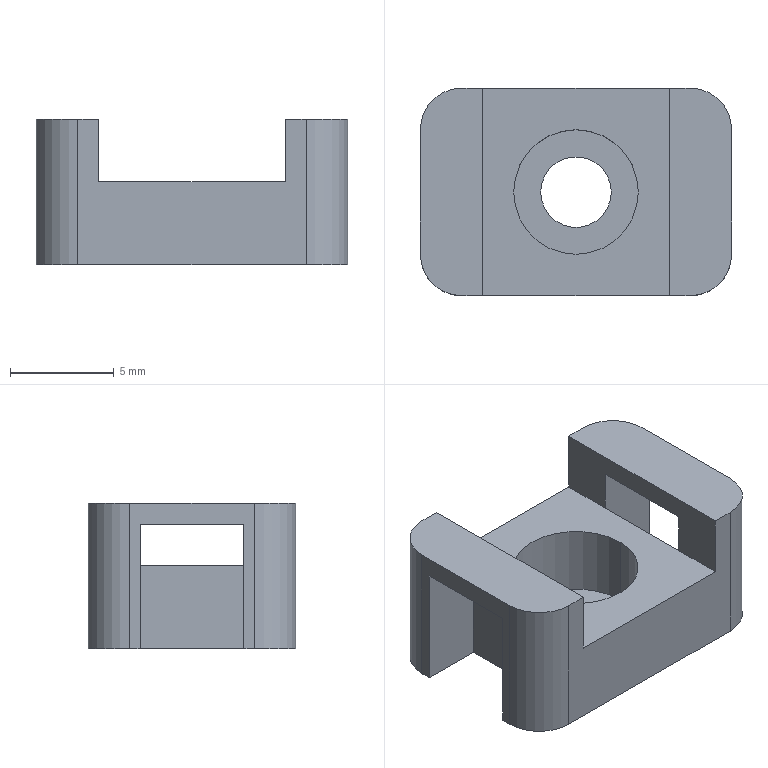Part | SolidWorks | features ICE 2, Extrusion 1, Fillet 1, HoleWzd 1 | 1 solid | 27 faces | box 15 x 10 x 7 mm | volume 474.384 mm3 | plane 19 | cylinder 8 | commonest cylinder face diameters 4 x4 3.4 x2 6 x2
STEP:
#1=CARTESIAN_POINT('',(-3.,0.,0.6));
#2=VERTEX_POINT('',#1);
#3=CARTESIAN_POINT('',(3.,0.,0.6));
#4=VERTEX_POINT('',#3);
#5=CARTESIAN_POINT('',(0.,0.,0.6));
#6=DIRECTION('',(0.,0.,1.));
#7=DIRECTION('',(1.,0.,0.));
#8=AXIS2_PLACEMENT_3D('',#5,#6,#7);
#9=CIRCLE('',#8,3.);
#10=EDGE_CURVE('',#2,#4,#9,.T.);
#11=ORIENTED_EDGE('',*,*,#10,.F.);
#12=CARTESIAN_POINT('',(-3.,0.,4.));
#13=VERTEX_POINT('',#12);
#14=CARTESIAN_POINT('',(-3.,0.,4.));
#15=DIRECTION('',(0.,0.,1.));
#16=VECTOR('',#15,1000.);
#17=LINE('',#14,#16);
#18=EDGE_CURVE('',#2,#13,#17,.T.);
#19=ORIENTED_EDGE('',*,*,#18,.T.);
#20=CARTESIAN_POINT('',(3.,0.,4.));
#21=VERTEX_POINT('',#20);
#22=CARTESIAN_POINT('',(0.,0.,4.));
#23=DIRECTION('',(0.,0.,1.));
#24=DIRECTION('',(1.,0.,0.));
#25=AXIS2_PLACEMENT_3D('',#22,#23,#24);
#26=CIRCLE('',#25,3.);
#27=EDGE_CURVE('',#13,#21,#26,.T.);
#28=ORIENTED_EDGE('',*,*,#27,.T.);
#29=CARTESIAN_POINT('',(3.,0.,4.));
#30=DIRECTION('',(0.,0.,1.));
#31=VECTOR('',#30,1000.);
#32=LINE('',#29,#31);
#33=EDGE_CURVE('',#4,#21,#32,.T.);
#34=ORIENTED_EDGE('',*,*,#33,.F.);
#35=EDGE_LOOP('',(#11,#19,#28,#34));
#36=FACE_OUTER_BOUND('',#35,.T.);
#37=CARTESIAN_POINT('',(0.,0.,4.));
#38=DIRECTION('',(0.,0.,1.));
#39=DIRECTION('',(1.,0.,0.));
#40=AXIS2_PLACEMENT_3D('',#37,#38,#39);
#41=CYLINDRICAL_SURFACE('',#40,3.);
#42=ADVANCED_FACE('',(#36),#41,.F.);
#43=CARTESIAN_POINT('',(-1.7,0.,0.));
#44=VERTEX_POINT('',#43);
#45=CARTESIAN_POINT('',(1.7,0.,0.));
#46=VERTEX_POINT('',#45);
#47=CARTESIAN_POINT('',(0.,0.,0.));
#48=DIRECTION('',(0.,0.,1.));
#49=DIRECTION('',(1.,0.,0.));
#50=AXIS2_PLACEMENT_3D('',#47,#48,#49);
#51=CIRCLE('',#50,1.7);
#52=EDGE_CURVE('',#44,#46,#51,.T.);
#53=ORIENTED_EDGE('',*,*,#52,.F.);
#54=CARTESIAN_POINT('',(-1.7,0.,0.6));
#55=VERTEX_POINT('',#54);
#56=CARTESIAN_POINT('',(-1.7,0.,4.));
#57=DIRECTION('',(0.,0.,1.));
#58=VECTOR('',#57,1000.);
#59=LINE('',#56,#58);
#60=EDGE_CURVE('',#44,#55,#59,.T.);
#61=ORIENTED_EDGE('',*,*,#60,.T.);
#62=CARTESIAN_POINT('',(1.7,0.,0.6));
#63=VERTEX_POINT('',#62);
#64=CARTESIAN_POINT('',(0.,0.,0.6));
#65=DIRECTION('',(0.,0.,1.));
#66=DIRECTION('',(1.,0.,0.));
#67=AXIS2_PLACEMENT_3D('',#64,#65,#66);
#68=CIRCLE('',#67,1.7);
#69=EDGE_CURVE('',#55,#63,#68,.T.);
#70=ORIENTED_EDGE('',*,*,#69,.T.);
#71=CARTESIAN_POINT('',(1.7,0.,4.));
#72=DIRECTION('',(0.,0.,1.));
#73=VECTOR('',#72,1000.);
#74=LINE('',#71,#73);
#75=EDGE_CURVE('',#46,#63,#74,.T.);
#76=ORIENTED_EDGE('',*,*,#75,.F.);
#77=EDGE_LOOP('',(#53,#61,#70,#76));
#78=FACE_OUTER_BOUND('',#77,.T.);
#79=CARTESIAN_POINT('',(0.,0.,4.));
#80=DIRECTION('',(0.,0.,1.));
#81=DIRECTION('',(1.,0.,0.));
#82=AXIS2_PLACEMENT_3D('',#79,#80,#81);
#83=CYLINDRICAL_SURFACE('',#82,1.7);
#84=ADVANCED_FACE('',(#78),#83,.F.);
#85=CARTESIAN_POINT('',(7.5,-3.,7.));
#86=VERTEX_POINT('',#85);
#87=CARTESIAN_POINT('',(7.5,3.,7.));
#88=VERTEX_POINT('',#87);
#89=CARTESIAN_POINT('',(7.5,-5.,7.));
#90=DIRECTION('',(0.,1.,0.));
#91=VECTOR('',#90,1000.);
#92=LINE('',#89,#91);
#93=EDGE_CURVE('',#86,#88,#92,.T.);
#94=ORIENTED_EDGE('',*,*,#93,.T.);
#95=CARTESIAN_POINT('',(5.5,5.,7.));
#96=VERTEX_POINT('',#95);
#97=CARTESIAN_POINT('',(5.5,3.,7.));
#98=DIRECTION('',(0.,0.,1.));
#99=DIRECTION('',(-1.,0.,0.));
#100=AXIS2_PLACEMENT_3D('',#97,#98,#99);
#101=CIRCLE('',#100,2.);
#102=EDGE_CURVE('',#88,#96,#101,.T.);
#103=ORIENTED_EDGE('',*,*,#102,.T.);
#104=CARTESIAN_POINT('',(4.5,5.,7.));
#105=VERTEX_POINT('',#104);
#106=CARTESIAN_POINT('',(-7.5,5.,7.));
#107=DIRECTION('',(-1.,0.,0.));
#108=VECTOR('',#107,1000.);
#109=LINE('',#106,#108);
#110=EDGE_CURVE('',#96,#105,#109,.T.);
#111=ORIENTED_EDGE('',*,*,#110,.T.);
#112=CARTESIAN_POINT('',(4.5,-5.,7.));
#113=VERTEX_POINT('',#112);
#114=CARTESIAN_POINT('',(4.5,0.,7.));
#115=DIRECTION('',(0.,-1.,0.));
#116=VECTOR('',#115,1000.);
#117=LINE('',#114,#116);
#118=EDGE_CURVE('',#105,#113,#117,.T.);
#119=ORIENTED_EDGE('',*,*,#118,.T.);
#120=CARTESIAN_POINT('',(5.5,-5.,7.));
#121=VERTEX_POINT('',#120);
#122=CARTESIAN_POINT('',(-7.5,-5.,7.));
#123=DIRECTION('',(1.,0.,0.));
#124=VECTOR('',#123,1000.);
#125=LINE('',#122,#124);
#126=EDGE_CURVE('',#113,#121,#125,.T.);
#127=ORIENTED_EDGE('',*,*,#126,.T.);
#128=CARTESIAN_POINT('',(5.5,-3.,7.));
#129=DIRECTION('',(0.,0.,1.));
#130=DIRECTION('',(-1.,0.,0.));
#131=AXIS2_PLACEMENT_3D('',#128,#129,#130);
#132=CIRCLE('',#131,2.);
#133=EDGE_CURVE('',#121,#86,#132,.T.);
#134=ORIENTED_EDGE('',*,*,#133,.T.);
#135=EDGE_LOOP('',(#94,#103,#111,#119,#127,#134));
#136=FACE_OUTER_BOUND('',#135,.T.);
#137=CARTESIAN_POINT('',(0.,0.,7.));
#138=DIRECTION('',(0.,0.,-1.));
#139=DIRECTION('',(-1.,0.,0.));
#140=AXIS2_PLACEMENT_3D('',#137,#138,#139);
#141=PLANE('',#140);
#142=ADVANCED_FACE('',(#136),#141,.F.);
#143=CARTESIAN_POINT('',(7.5,2.5,0.));
#144=VERTEX_POINT('',#143);
#145=CARTESIAN_POINT('',(7.5,3.,0.));
#146=VERTEX_POINT('',#145);
#147=CARTESIAN_POINT('',(7.5,-5.,0.));
#148=DIRECTION('',(0.,1.,0.));
#149=VECTOR('',#148,1000.);
#150=LINE('',#147,#149);
#151=EDGE_CURVE('',#144,#146,#150,.T.);
#152=ORIENTED_EDGE('',*,*,#151,.T.);
#153=CARTESIAN_POINT('',(7.5,3.,7.));
#154=DIRECTION('',(0.,0.,1.));
#155=VECTOR('',#154,1000.);
#156=LINE('',#153,#155);
#157=EDGE_CURVE('',#146,#88,#156,.T.);
#158=ORIENTED_EDGE('',*,*,#157,.T.);
#159=ORIENTED_EDGE('',*,*,#93,.F.);
#160=CARTESIAN_POINT('',(7.5,-3.,0.));
#161=VERTEX_POINT('',#160);
#162=CARTESIAN_POINT('',(7.5,-3.,7.));
#163=DIRECTION('',(0.,0.,-1.));
#164=VECTOR('',#163,1000.);
#165=LINE('',#162,#164);
#166=EDGE_CURVE('',#86,#161,#165,.T.);
#167=ORIENTED_EDGE('',*,*,#166,.T.);
#168=CARTESIAN_POINT('',(7.5,-2.5,0.));
#169=VERTEX_POINT('',#168);
#170=CARTESIAN_POINT('',(7.5,-5.,0.));
#171=DIRECTION('',(0.,1.,0.));
#172=VECTOR('',#171,1000.);
#173=LINE('',#170,#172);
#174=EDGE_CURVE('',#161,#169,#173,.T.);
#175=ORIENTED_EDGE('',*,*,#174,.T.);
#176=CARTESIAN_POINT('',(7.5,-2.5,6.));
#177=VERTEX_POINT('',#176);
#178=CARTESIAN_POINT('',(7.5,-2.5,7.));
#179=DIRECTION('',(0.,0.,1.));
#180=VECTOR('',#179,1000.);
#181=LINE('',#178,#180);
#182=EDGE_CURVE('',#169,#177,#181,.T.);
#183=ORIENTED_EDGE('',*,*,#182,.T.);
#184=CARTESIAN_POINT('',(7.5,2.5,6.));
#185=VERTEX_POINT('',#184);
#186=CARTESIAN_POINT('',(7.5,-5.,6.));
#187=DIRECTION('',(0.,1.,0.));
#188=VECTOR('',#187,1000.);
#189=LINE('',#186,#188);
#190=EDGE_CURVE('',#177,#185,#189,.T.);
#191=ORIENTED_EDGE('',*,*,#190,.T.);
#192=CARTESIAN_POINT('',(7.5,2.5,7.));
#193=DIRECTION('',(0.,0.,-1.));
#194=VECTOR('',#193,1000.);
#195=LINE('',#192,#194);
#196=EDGE_CURVE('',#185,#144,#195,.T.);
#197=ORIENTED_EDGE('',*,*,#196,.T.);
#198=EDGE_LOOP('',(#152,#158,#159,#167,#175,#183,#191,#197));
#199=FACE_OUTER_BOUND('',#198,.T.);
#200=CARTESIAN_POINT('',(7.5,-5.,7.));
#201=DIRECTION('',(-1.,0.,0.));
#202=DIRECTION('',(0.,0.,1.));
#203=AXIS2_PLACEMENT_3D('',#200,#201,#202);
#204=PLANE('',#203);
#205=ADVANCED_FACE('',(#199),#204,.F.);
#206=CARTESIAN_POINT('',(5.5,5.,0.));
#207=VERTEX_POINT('',#206);
#208=CARTESIAN_POINT('',(-5.5,5.,0.));
#209=VERTEX_POINT('',#208);
#210=CARTESIAN_POINT('',(-7.5,5.,0.));
#211=DIRECTION('',(-1.,0.,0.));
#212=VECTOR('',#211,1000.);
#213=LINE('',#210,#212);
#214=EDGE_CURVE('',#207,#209,#213,.T.);
#215=ORIENTED_EDGE('',*,*,#214,.T.);
#216=CARTESIAN_POINT('',(-5.5,5.,7.));
#217=VERTEX_POINT('',#216);
#218=CARTESIAN_POINT('',(-5.5,5.,7.));
#219=DIRECTION('',(0.,0.,1.));
#220=VECTOR('',#219,1000.);
#221=LINE('',#218,#220);
#222=EDGE_CURVE('',#209,#217,#221,.T.);
#223=ORIENTED_EDGE('',*,*,#222,.T.);
#224=CARTESIAN_POINT('',(-4.5,5.,7.));
#225=VERTEX_POINT('',#224);
#226=CARTESIAN_POINT('',(-7.5,5.,7.));
#227=DIRECTION('',(-1.,0.,0.));
#228=VECTOR('',#227,1000.);
#229=LINE('',#226,#228);
#230=EDGE_CURVE('',#225,#217,#229,.T.);
#231=ORIENTED_EDGE('',*,*,#230,.F.);
#232=CARTESIAN_POINT('',(-4.5,5.,4.));
#233=VERTEX_POINT('',#232);
#234=CARTESIAN_POINT('',(-4.5,5.,7.));
#235=DIRECTION('',(0.,0.,-1.));
#236=VECTOR('',#235,1000.);
#237=LINE('',#234,#236);
#238=EDGE_CURVE('',#225,#233,#237,.T.);
#239=ORIENTED_EDGE('',*,*,#238,.T.);
#240=CARTESIAN_POINT('',(4.5,5.,4.));
#241=VERTEX_POINT('',#240);
#242=CARTESIAN_POINT('',(-7.5,5.,4.));
#243=DIRECTION('',(1.,0.,0.));
#244=VECTOR('',#243,1000.);
#245=LINE('',#242,#244);
#246=EDGE_CURVE('',#233,#241,#245,.T.);
#247=ORIENTED_EDGE('',*,*,#246,.T.);
#248=CARTESIAN_POINT('',(4.5,5.,7.));
#249=DIRECTION('',(0.,0.,1.));
#250=VECTOR('',#249,1000.);
#251=LINE('',#248,#250);
#252=EDGE_CURVE('',#241,#105,#251,.T.);
#253=ORIENTED_EDGE('',*,*,#252,.T.);
#254=ORIENTED_EDGE('',*,*,#110,.F.);
#255=CARTESIAN_POINT('',(5.5,5.,7.));
#256=DIRECTION('',(0.,0.,-1.));
#257=VECTOR('',#256,1000.);
#258=LINE('',#255,#257);
#259=EDGE_CURVE('',#96,#207,#258,.T.);
#260=ORIENTED_EDGE('',*,*,#259,.T.);
#261=EDGE_LOOP('',(#215,#223,#231,#239,#247,#253,#254,#260));
#262=FACE_OUTER_BOUND('',#261,.T.);
#263=CARTESIAN_POINT('',(-7.5,5.,7.));
#264=DIRECTION('',(0.,-1.,0.));
#265=DIRECTION('',(0.,0.,-1.));
#266=AXIS2_PLACEMENT_3D('',#263,#264,#265);
#267=PLANE('',#266);
#268=ADVANCED_FACE('',(#262),#267,.F.);
#269=CARTESIAN_POINT('',(-7.5,3.,7.));
#270=VERTEX_POINT('',#269);
#271=CARTESIAN_POINT('',(-7.5,-3.,7.));
#272=VERTEX_POINT('',#271);
#273=CARTESIAN_POINT('',(-7.5,-5.,7.));
#274=DIRECTION('',(0.,-1.,0.));
#275=VECTOR('',#274,1000.);
#276=LINE('',#273,#275);
#277=EDGE_CURVE('',#270,#272,#276,.T.);
#278=ORIENTED_EDGE('',*,*,#277,.F.);
#279=CARTESIAN_POINT('',(-7.5,3.,0.));
#280=VERTEX_POINT('',#279);
#281=CARTESIAN_POINT('',(-7.5,3.,7.));
#282=DIRECTION('',(0.,0.,-1.));
#283=VECTOR('',#282,1000.);
#284=LINE('',#281,#283);
#285=EDGE_CURVE('',#270,#280,#284,.T.);
#286=ORIENTED_EDGE('',*,*,#285,.T.);
#287=CARTESIAN_POINT('',(-7.5,2.5,0.));
#288=VERTEX_POINT('',#287);
#289=CARTESIAN_POINT('',(-7.5,-5.,0.));
#290=DIRECTION('',(0.,-1.,0.));
#291=VECTOR('',#290,1000.);
#292=LINE('',#289,#291);
#293=EDGE_CURVE('',#280,#288,#292,.T.);
#294=ORIENTED_EDGE('',*,*,#293,.T.);
#295=CARTESIAN_POINT('',(-7.5,2.5,6.));
#296=VERTEX_POINT('',#295);
#297=CARTESIAN_POINT('',(-7.5,2.5,7.));
#298=DIRECTION('',(0.,0.,1.));
#299=VECTOR('',#298,1000.);
#300=LINE('',#297,#299);
#301=EDGE_CURVE('',#288,#296,#300,.T.);
#302=ORIENTED_EDGE('',*,*,#301,.T.);
#303=CARTESIAN_POINT('',(-7.5,-2.5,6.));
#304=VERTEX_POINT('',#303);
#305=CARTESIAN_POINT('',(-7.5,-5.,6.));
#306=DIRECTION('',(0.,1.,0.));
#307=VECTOR('',#306,1000.);
#308=LINE('',#305,#307);
#309=EDGE_CURVE('',#304,#296,#308,.T.);
#310=ORIENTED_EDGE('',*,*,#309,.F.);
#311=CARTESIAN_POINT('',(-7.5,-2.5,0.));
#312=VERTEX_POINT('',#311);
#313=CARTESIAN_POINT('',(-7.5,-2.5,7.));
#314=DIRECTION('',(0.,0.,-1.));
#315=VECTOR('',#314,1000.);
#316=LINE('',#313,#315);
#317=EDGE_CURVE('',#304,#312,#316,.T.);
#318=ORIENTED_EDGE('',*,*,#317,.T.);
#319=CARTESIAN_POINT('',(-7.5,-3.,0.));
#320=VERTEX_POINT('',#319);
#321=CARTESIAN_POINT('',(-7.5,-5.,0.));
#322=DIRECTION('',(0.,-1.,0.));
#323=VECTOR('',#322,1000.);
#324=LINE('',#321,#323);
#325=EDGE_CURVE('',#312,#320,#324,.T.);
#326=ORIENTED_EDGE('',*,*,#325,.T.);
#327=CARTESIAN_POINT('',(-7.5,-3.,7.));
#328=DIRECTION('',(0.,0.,1.));
#329=VECTOR('',#328,1000.);
#330=LINE('',#327,#329);
#331=EDGE_CURVE('',#320,#272,#330,.T.);
#332=ORIENTED_EDGE('',*,*,#331,.T.);
#333=EDGE_LOOP('',(#278,#286,#294,#302,#310,#318,#326,#332));
#334=FACE_OUTER_BOUND('',#333,.T.);
#335=CARTESIAN_POINT('',(-7.5,-5.,7.));
#336=DIRECTION('',(1.,0.,0.));
#337=DIRECTION('',(0.,0.,-1.));
#338=AXIS2_PLACEMENT_3D('',#335,#336,#337);
#339=PLANE('',#338);
#340=ADVANCED_FACE('',(#334),#339,.F.);
#341=CARTESIAN_POINT('',(-5.5,-5.,7.));
#342=VERTEX_POINT('',#341);
#343=CARTESIAN_POINT('',(-4.5,-5.,7.));
#344=VERTEX_POINT('',#343);
#345=CARTESIAN_POINT('',(-7.5,-5.,7.));
#346=DIRECTION('',(1.,0.,0.));
#347=VECTOR('',#346,1000.);
#348=LINE('',#345,#347);
#349=EDGE_CURVE('',#342,#344,#348,.T.);
#350=ORIENTED_EDGE('',*,*,#349,.F.);
#351=CARTESIAN_POINT('',(-5.5,-5.,0.));
#352=VERTEX_POINT('',#351);
#353=CARTESIAN_POINT('',(-5.5,-5.,7.));
#354=DIRECTION('',(0.,0.,-1.));
#355=VECTOR('',#354,1000.);
#356=LINE('',#353,#355);
#357=EDGE_CURVE('',#342,#352,#356,.T.);
#358=ORIENTED_EDGE('',*,*,#357,.T.);
#359=CARTESIAN_POINT('',(5.5,-5.,0.));
#360=VERTEX_POINT('',#359);
#361=CARTESIAN_POINT('',(-7.5,-5.,0.));
#362=DIRECTION('',(1.,0.,0.));
#363=VECTOR('',#362,1000.);
#364=LINE('',#361,#363);
#365=EDGE_CURVE('',#352,#360,#364,.T.);
#366=ORIENTED_EDGE('',*,*,#365,.T.);
#367=CARTESIAN_POINT('',(5.5,-5.,7.));
#368=DIRECTION('',(0.,0.,1.));
#369=VECTOR('',#368,1000.);
#370=LINE('',#367,#369);
#371=EDGE_CURVE('',#360,#121,#370,.T.);
#372=ORIENTED_EDGE('',*,*,#371,.T.);
#373=ORIENTED_EDGE('',*,*,#126,.F.);
#374=CARTESIAN_POINT('',(4.5,-5.,4.));
#375=VERTEX_POINT('',#374);
#376=CARTESIAN_POINT('',(4.5,-5.,7.));
#377=DIRECTION('',(0.,0.,-1.));
#378=VECTOR('',#377,1000.);
#379=LINE('',#376,#378);
#380=EDGE_CURVE('',#113,#375,#379,.T.);
#381=ORIENTED_EDGE('',*,*,#380,.T.);
#382=CARTESIAN_POINT('',(-4.5,-5.,4.));
#383=VERTEX_POINT('',#382);
#384=CARTESIAN_POINT('',(-7.5,-5.,4.));
#385=DIRECTION('',(-1.,0.,0.));
#386=VECTOR('',#385,1000.);
#387=LINE('',#384,#386);
#388=EDGE_CURVE('',#375,#383,#387,.T.);
#389=ORIENTED_EDGE('',*,*,#388,.T.);
#390=CARTESIAN_POINT('',(-4.5,-5.,7.));
#391=DIRECTION('',(0.,0.,1.));
#392=VECTOR('',#391,1000.);
#393=LINE('',#390,#392);
#394=EDGE_CURVE('',#383,#344,#393,.T.);
#395=ORIENTED_EDGE('',*,*,#394,.T.);
#396=EDGE_LOOP('',(#350,#358,#366,#372,#373,#381,#389,#395));
#397=FACE_OUTER_BOUND('',#396,.T.);
#398=CARTESIAN_POINT('',(-7.5,-5.,7.));
#399=DIRECTION('',(0.,1.,0.));
#400=DIRECTION('',(0.,0.,1.));
#401=AXIS2_PLACEMENT_3D('',#398,#399,#400);
#402=PLANE('',#401);
#403=ADVANCED_FACE('',(#397),#402,.F.);
#404=ORIENTED_EDGE('',*,*,#230,.T.);
#405=CARTESIAN_POINT('',(-5.5,3.,7.));
#406=DIRECTION('',(0.,0.,1.));
#407=DIRECTION('',(-1.,0.,0.));
#408=AXIS2_PLACEMENT_3D('',#405,#406,#407);
#409=CIRCLE('',#408,2.);
#410=EDGE_CURVE('',#217,#270,#409,.T.);
#411=ORIENTED_EDGE('',*,*,#410,.T.);
#412=ORIENTED_EDGE('',*,*,#277,.T.);
#413=CARTESIAN_POINT('',(-5.5,-3.,7.));
#414=DIRECTION('',(0.,0.,1.));
#415=DIRECTION('',(-1.,0.,0.));
#416=AXIS2_PLACEMENT_3D('',#413,#414,#415);
#417=CIRCLE('',#416,2.);
#418=EDGE_CURVE('',#272,#342,#417,.T.);
#419=ORIENTED_EDGE('',*,*,#418,.T.);
#420=ORIENTED_EDGE('',*,*,#349,.T.);
#421=CARTESIAN_POINT('',(-4.5,0.,7.));
#422=DIRECTION('',(0.,1.,0.));
#423=VECTOR('',#422,1000.);
#424=LINE('',#421,#423);
#425=EDGE_CURVE('',#344,#225,#424,.T.);
#426=ORIENTED_EDGE('',*,*,#425,.T.);
#427=EDGE_LOOP('',(#404,#411,#412,#419,#420,#426));
#428=FACE_OUTER_BOUND('',#427,.T.);
#429=CARTESIAN_POINT('',(0.,0.,7.));
#430=DIRECTION('',(0.,0.,-1.));
#431=DIRECTION('',(-1.,0.,0.));
#432=AXIS2_PLACEMENT_3D('',#429,#430,#431);
#433=PLANE('',#432);
#434=ADVANCED_FACE('',(#428),#433,.F.);
#435=CARTESIAN_POINT('',(0.,0.,0.));
#436=DIRECTION('',(0.,0.,1.));
#437=DIRECTION('',(1.,0.,0.));
#438=AXIS2_PLACEMENT_3D('',#435,#436,#437);
#439=CIRCLE('',#438,1.7);
#440=EDGE_CURVE('',#46,#44,#439,.T.);
#441=ORIENTED_EDGE('',*,*,#440,.T.);
#442=ORIENTED_EDGE('',*,*,#52,.T.);
#443=EDGE_LOOP('',(#441,#442));
#444=FACE_BOUND('',#443,.T.);
#445=ORIENTED_EDGE('',*,*,#293,.F.);
#446=CARTESIAN_POINT('',(-5.5,3.,0.));
#447=DIRECTION('',(0.,0.,-1.));
#448=DIRECTION('',(-1.,0.,0.));
#449=AXIS2_PLACEMENT_3D('',#446,#447,#448);
#450=CIRCLE('',#449,2.);
#451=EDGE_CURVE('',#280,#209,#450,.T.);
#452=ORIENTED_EDGE('',*,*,#451,.T.);
#453=ORIENTED_EDGE('',*,*,#214,.F.);
#454=CARTESIAN_POINT('',(5.5,3.,0.));
#455=DIRECTION('',(0.,0.,-1.));
#456=DIRECTION('',(-1.,0.,0.));
#457=AXIS2_PLACEMENT_3D('',#454,#455,#456);
#458=CIRCLE('',#457,2.);
#459=EDGE_CURVE('',#207,#146,#458,.T.);
#460=ORIENTED_EDGE('',*,*,#459,.T.);
#461=ORIENTED_EDGE('',*,*,#151,.F.);
#462=CARTESIAN_POINT('',(4.5,2.5,0.));
#463=VERTEX_POINT('',#462);
#464=CARTESIAN_POINT('',(10.5,2.5,0.));
#465=DIRECTION('',(1.,0.,0.));
#466=VECTOR('',#465,1000.);
#467=LINE('',#464,#466);
#468=EDGE_CURVE('',#463,#144,#467,.T.);
#469=ORIENTED_EDGE('',*,*,#468,.F.);
#470=CARTESIAN_POINT('',(4.5,-2.5,0.));
#471=VERTEX_POINT('',#470);
#472=CARTESIAN_POINT('',(4.5,-2.5,0.));
#473=DIRECTION('',(0.,1.,0.));
#474=VECTOR('',#473,1000.);
#475=LINE('',#472,#474);
#476=EDGE_CURVE('',#471,#463,#475,.T.);
#477=ORIENTED_EDGE('',*,*,#476,.F.);
#478=CARTESIAN_POINT('',(10.5,-2.5,0.));
#479=DIRECTION('',(-1.,0.,0.));
#480=VECTOR('',#479,1000.);
#481=LINE('',#478,#480);
#482=EDGE_CURVE('',#169,#471,#481,.T.);
#483=ORIENTED_EDGE('',*,*,#482,.F.);
#484=ORIENTED_EDGE('',*,*,#174,.F.);
#485=CARTESIAN_POINT('',(5.5,-3.,0.));
#486=DIRECTION('',(0.,0.,-1.));
#487=DIRECTION('',(-1.,0.,0.));
#488=AXIS2_PLACEMENT_3D('',#485,#486,#487);
#489=CIRCLE('',#488,2.);
#490=EDGE_CURVE('',#161,#360,#489,.T.);
#491=ORIENTED_EDGE('',*,*,#490,.T.);
#492=ORIENTED_EDGE('',*,*,#365,.F.);
#493=CARTESIAN_POINT('',(-5.5,-3.,0.));
#494=DIRECTION('',(0.,0.,-1.));
#495=DIRECTION('',(-1.,0.,0.));
#496=AXIS2_PLACEMENT_3D('',#493,#494,#495);
#497=CIRCLE('',#496,2.);
#498=EDGE_CURVE('',#352,#320,#497,.T.);
#499=ORIENTED_EDGE('',*,*,#498,.T.);
#500=ORIENTED_EDGE('',*,*,#325,.F.);
#501=CARTESIAN_POINT('',(-4.5,-2.5,0.));
#502=VERTEX_POINT('',#501);
#503=CARTESIAN_POINT('',(-10.5,-2.5,0.));
#504=DIRECTION('',(-1.,0.,0.));
#505=VECTOR('',#504,1000.);
#506=LINE('',#503,#505);
#507=EDGE_CURVE('',#502,#312,#506,.T.);
#508=ORIENTED_EDGE('',*,*,#507,.F.);
#509=CARTESIAN_POINT('',(-4.5,2.5,0.));
#510=VERTEX_POINT('',#509);
#511=CARTESIAN_POINT('',(-4.5,-2.5,0.));
#512=DIRECTION('',(0.,-1.,0.));
#513=VECTOR('',#512,1000.);
#514=LINE('',#511,#513);
#515=EDGE_CURVE('',#510,#502,#514,.T.);
#516=ORIENTED_EDGE('',*,*,#515,.F.);
#517=CARTESIAN_POINT('',(-10.5,2.5,0.));
#518=DIRECTION('',(1.,0.,0.));
#519=VECTOR('',#518,1000.);
#520=LINE('',#517,#519);
#521=EDGE_CURVE('',#288,#510,#520,.T.);
#522=ORIENTED_EDGE('',*,*,#521,.F.);
#523=EDGE_LOOP('',(#445,#452,#453,#460,#461,#469,#477,#483,#484,#491,#492,#499,#500,#508,#516,#522));
#524=FACE_OUTER_BOUND('',#523,.T.);
#525=CARTESIAN_POINT('',(0.,0.,0.));
#526=DIRECTION('',(0.,0.,-1.));
#527=DIRECTION('',(-1.,0.,0.));
#528=AXIS2_PLACEMENT_3D('',#525,#526,#527);
#529=PLANE('',#528);
#530=ADVANCED_FACE('',(#444,#524),#529,.T.);
#531=CARTESIAN_POINT('',(0.,0.,4.));
#532=DIRECTION('',(0.,0.,1.));
#533=DIRECTION('',(1.,0.,0.));
#534=AXIS2_PLACEMENT_3D('',#531,#532,#533);
#535=CIRCLE('',#534,3.);
#536=EDGE_CURVE('',#21,#13,#535,.T.);
#537=ORIENTED_EDGE('',*,*,#536,.F.);
#538=ORIENTED_EDGE('',*,*,#27,.F.);
#539=EDGE_LOOP('',(#537,#538));
#540=FACE_BOUND('',#539,.T.);
#541=CARTESIAN_POINT('',(-4.5,2.5,4.));
#542=VERTEX_POINT('',#541);
#543=CARTESIAN_POINT('',(-4.5,-7.884,4.));
#544=DIRECTION('',(0.,-1.,0.));
#545=VECTOR('',#544,1000.);
#546=LINE('',#543,#545);
#547=EDGE_CURVE('',#233,#542,#546,.T.);
#548=ORIENTED_EDGE('',*,*,#547,.T.);
#549=CARTESIAN_POINT('',(-4.5,-2.5,4.));
#550=VERTEX_POINT('',#549);
#551=CARTESIAN_POINT('',(-4.5,-7.884,4.));
#552=DIRECTION('',(0.,-1.,0.));
#553=VECTOR('',#552,1000.);
#554=LINE('',#551,#553);
#555=EDGE_CURVE('',#542,#550,#554,.T.);
#556=ORIENTED_EDGE('',*,*,#555,.T.);
#557=CARTESIAN_POINT('',(-4.5,-7.884,4.));
#558=DIRECTION('',(0.,-1.,0.));
#559=VECTOR('',#558,1000.);
#560=LINE('',#557,#559);
#561=EDGE_CURVE('',#550,#383,#560,.T.);
#562=ORIENTED_EDGE('',*,*,#561,.T.);
#563=ORIENTED_EDGE('',*,*,#388,.F.);
#564=CARTESIAN_POINT('',(4.5,-2.5,4.));
#565=VERTEX_POINT('',#564);
#566=CARTESIAN_POINT('',(4.5,-7.884,4.));
#567=DIRECTION('',(0.,1.,0.));
#568=VECTOR('',#567,1000.);
#569=LINE('',#566,#568);
#570=EDGE_CURVE('',#375,#565,#569,.T.);
#571=ORIENTED_EDGE('',*,*,#570,.T.);
#572=CARTESIAN_POINT('',(4.5,2.5,4.));
#573=VERTEX_POINT('',#572);
#574=CARTESIAN_POINT('',(4.5,-7.884,4.));
#575=DIRECTION('',(0.,1.,0.));
#576=VECTOR('',#575,1000.);
#577=LINE('',#574,#576);
#578=EDGE_CURVE('',#565,#573,#577,.T.);
#579=ORIENTED_EDGE('',*,*,#578,.T.);
#580=CARTESIAN_POINT('',(4.5,-7.884,4.));
#581=DIRECTION('',(0.,1.,0.));
#582=VECTOR('',#581,1000.);
#583=LINE('',#580,#582);
#584=EDGE_CURVE('',#573,#241,#583,.T.);
#585=ORIENTED_EDGE('',*,*,#584,.T.);
#586=ORIENTED_EDGE('',*,*,#246,.F.);
#587=EDGE_LOOP('',(#548,#556,#562,#563,#571,#579,#585,#586));
#588=FACE_OUTER_BOUND('',#587,.T.);
#589=CARTESIAN_POINT('',(0.,0.,4.));
#590=DIRECTION('',(0.,0.,-1.));
#591=DIRECTION('',(-1.,0.,0.));
#592=AXIS2_PLACEMENT_3D('',#589,#590,#591);
#593=PLANE('',#592);
#594=ADVANCED_FACE('',(#540,#588),#593,.F.);
#595=CARTESIAN_POINT('',(4.5,-2.5,6.));
#596=VERTEX_POINT('',#595);
#597=CARTESIAN_POINT('',(4.5,2.5,6.));
#598=VERTEX_POINT('',#597);
#599=CARTESIAN_POINT('',(4.5,-2.5,6.));
#600=DIRECTION('',(0.,1.,0.));
#601=VECTOR('',#600,1000.);
#602=LINE('',#599,#601);
#603=EDGE_CURVE('',#596,#598,#602,.T.);
#604=ORIENTED_EDGE('',*,*,#603,.F.);
#605=CARTESIAN_POINT('',(4.5,-2.5,6.));
#606=DIRECTION('',(0.,0.,-1.));
#607=VECTOR('',#606,1000.);
#608=LINE('',#605,#607);
#609=EDGE_CURVE('',#596,#565,#608,.T.);
#610=ORIENTED_EDGE('',*,*,#609,.T.);
#611=ORIENTED_EDGE('',*,*,#570,.F.);
#612=ORIENTED_EDGE('',*,*,#380,.F.);
#613=ORIENTED_EDGE('',*,*,#118,.F.);
#614=ORIENTED_EDGE('',*,*,#252,.F.);
#615=ORIENTED_EDGE('',*,*,#584,.F.);
#616=CARTESIAN_POINT('',(4.5,2.5,6.));
#617=DIRECTION('',(0.,0.,-1.));
#618=VECTOR('',#617,1000.);
#619=LINE('',#616,#618);
#620=EDGE_CURVE('',#598,#573,#619,.T.);
#621=ORIENTED_EDGE('',*,*,#620,.F.);
#622=EDGE_LOOP('',(#604,#610,#611,#612,#613,#614,#615,#621));
#623=FACE_OUTER_BOUND('',#622,.T.);
#624=CARTESIAN_POINT('',(4.5,-7.884,4.));
#625=DIRECTION('',(1.,0.,0.));
#626=DIRECTION('',(0.,0.,-1.));
#627=AXIS2_PLACEMENT_3D('',#624,#625,#626);
#628=PLANE('',#627);
#629=ADVANCED_FACE('',(#623),#628,.F.);
#630=CARTESIAN_POINT('',(-4.5,2.5,6.));
#631=VERTEX_POINT('',#630);
#632=CARTESIAN_POINT('',(-4.5,-2.5,6.));
#633=VERTEX_POINT('',#632);
#634=CARTESIAN_POINT('',(-4.5,-2.5,6.));
#635=DIRECTION('',(0.,-1.,0.));
#636=VECTOR('',#635,1000.);
#637=LINE('',#634,#636);
#638=EDGE_CURVE('',#631,#633,#637,.T.);
#639=ORIENTED_EDGE('',*,*,#638,.F.);
#640=CARTESIAN_POINT('',(-4.5,2.5,6.));
#641=DIRECTION('',(0.,0.,-1.));
#642=VECTOR('',#641,1000.);
#643=LINE('',#640,#642);
#644=EDGE_CURVE('',#631,#542,#643,.T.);
#645=ORIENTED_EDGE('',*,*,#644,.T.);
#646=ORIENTED_EDGE('',*,*,#547,.F.);
#647=ORIENTED_EDGE('',*,*,#238,.F.);
#648=ORIENTED_EDGE('',*,*,#425,.F.);
#649=ORIENTED_EDGE('',*,*,#394,.F.);
#650=ORIENTED_EDGE('',*,*,#561,.F.);
#651=CARTESIAN_POINT('',(-4.5,-2.5,6.));
#652=DIRECTION('',(0.,0.,-1.));
#653=VECTOR('',#652,1000.);
#654=LINE('',#651,#653);
#655=EDGE_CURVE('',#633,#550,#654,.T.);
#656=ORIENTED_EDGE('',*,*,#655,.F.);
#657=EDGE_LOOP('',(#639,#645,#646,#647,#648,#649,#650,#656));
#658=FACE_OUTER_BOUND('',#657,.T.);
#659=CARTESIAN_POINT('',(-4.5,-7.884,4.));
#660=DIRECTION('',(-1.,0.,0.));
#661=DIRECTION('',(0.,0.,1.));
#662=AXIS2_PLACEMENT_3D('',#659,#660,#661);
#663=PLANE('',#662);
#664=ADVANCED_FACE('',(#658),#663,.F.);
#665=CARTESIAN_POINT('',(4.5,-2.5,6.));
#666=DIRECTION('',(0.,0.,-1.));
#667=VECTOR('',#666,1000.);
#668=LINE('',#665,#667);
#669=EDGE_CURVE('',#565,#471,#668,.T.);
#670=ORIENTED_EDGE('',*,*,#669,.T.);
#671=ORIENTED_EDGE('',*,*,#476,.T.);
#672=CARTESIAN_POINT('',(4.5,2.5,6.));
#673=DIRECTION('',(0.,0.,-1.));
#674=VECTOR('',#673,1000.);
#675=LINE('',#672,#674);
#676=EDGE_CURVE('',#573,#463,#675,.T.);
#677=ORIENTED_EDGE('',*,*,#676,.F.);
#678=ORIENTED_EDGE('',*,*,#578,.F.);
#679=EDGE_LOOP('',(#670,#671,#677,#678));
#680=FACE_OUTER_BOUND('',#679,.T.);
#681=CARTESIAN_POINT('',(4.5,-2.5,6.));
#682=DIRECTION('',(-1.,0.,0.));
#683=DIRECTION('',(0.,0.,1.));
#684=AXIS2_PLACEMENT_3D('',#681,#682,#683);
#685=PLANE('',#684);
#686=ADVANCED_FACE('',(#680),#685,.F.);
#687=ORIENTED_EDGE('',*,*,#482,.T.);
#688=ORIENTED_EDGE('',*,*,#669,.F.);
#689=ORIENTED_EDGE('',*,*,#609,.F.);
#690=CARTESIAN_POINT('',(10.5,-2.5,6.));
#691=DIRECTION('',(-1.,0.,0.));
#692=VECTOR('',#691,1000.);
#693=LINE('',#690,#692);
#694=EDGE_CURVE('',#177,#596,#693,.T.);
#695=ORIENTED_EDGE('',*,*,#694,.F.);
#696=ORIENTED_EDGE('',*,*,#182,.F.);
#697=EDGE_LOOP('',(#687,#688,#689,#695,#696));
#698=FACE_OUTER_BOUND('',#697,.T.);
#699=CARTESIAN_POINT('',(10.5,-2.5,6.));
#700=DIRECTION('',(0.,-1.,0.));
#701=DIRECTION('',(0.,0.,-1.));
#702=AXIS2_PLACEMENT_3D('',#699,#700,#701);
#703=PLANE('',#702);
#704=ADVANCED_FACE('',(#698),#703,.F.);
#705=CARTESIAN_POINT('',(10.5,2.5,6.));
#706=DIRECTION('',(1.,0.,0.));
#707=VECTOR('',#706,1000.);
#708=LINE('',#705,#707);
#709=EDGE_CURVE('',#598,#185,#708,.T.);
#710=ORIENTED_EDGE('',*,*,#709,.F.);
#711=ORIENTED_EDGE('',*,*,#620,.T.);
#712=ORIENTED_EDGE('',*,*,#676,.T.);
#713=ORIENTED_EDGE('',*,*,#468,.T.);
#714=ORIENTED_EDGE('',*,*,#196,.F.);
#715=EDGE_LOOP('',(#710,#711,#712,#713,#714));
#716=FACE_OUTER_BOUND('',#715,.T.);
#717=CARTESIAN_POINT('',(10.5,2.5,6.));
#718=DIRECTION('',(0.,1.,0.));
#719=DIRECTION('',(0.,0.,1.));
#720=AXIS2_PLACEMENT_3D('',#717,#718,#719);
#721=PLANE('',#720);
#722=ADVANCED_FACE('',(#716),#721,.F.);
#723=ORIENTED_EDGE('',*,*,#694,.T.);
#724=ORIENTED_EDGE('',*,*,#603,.T.);
#725=ORIENTED_EDGE('',*,*,#709,.T.);
#726=ORIENTED_EDGE('',*,*,#190,.F.);
#727=EDGE_LOOP('',(#723,#724,#725,#726));
#728=FACE_OUTER_BOUND('',#727,.T.);
#729=CARTESIAN_POINT('',(0.,0.,6.));
#730=DIRECTION('',(0.,0.,1.));
#731=DIRECTION('',(1.,0.,0.));
#732=AXIS2_PLACEMENT_3D('',#729,#730,#731);
#733=PLANE('',#732);
#734=ADVANCED_FACE('',(#728),#733,.F.);
#735=CARTESIAN_POINT('',(-4.5,2.5,6.));
#736=DIRECTION('',(0.,0.,-1.));
#737=VECTOR('',#736,1000.);
#738=LINE('',#735,#737);
#739=EDGE_CURVE('',#542,#510,#738,.T.);
#740=ORIENTED_EDGE('',*,*,#739,.T.);
#741=ORIENTED_EDGE('',*,*,#515,.T.);
#742=CARTESIAN_POINT('',(-4.5,-2.5,6.));
#743=DIRECTION('',(0.,0.,-1.));
#744=VECTOR('',#743,1000.);
#745=LINE('',#742,#744);
#746=EDGE_CURVE('',#550,#502,#745,.T.);
#747=ORIENTED_EDGE('',*,*,#746,.F.);
#748=ORIENTED_EDGE('',*,*,#555,.F.);
#749=EDGE_LOOP('',(#740,#741,#747,#748));
#750=FACE_OUTER_BOUND('',#749,.T.);
#751=CARTESIAN_POINT('',(-4.5,-2.5,6.));
#752=DIRECTION('',(1.,0.,0.));
#753=DIRECTION('',(0.,1.,0.));
#754=AXIS2_PLACEMENT_3D('',#751,#752,#753);
#755=PLANE('',#754);
#756=ADVANCED_FACE('',(#750),#755,.F.);
#757=ORIENTED_EDGE('',*,*,#521,.T.);
#758=ORIENTED_EDGE('',*,*,#739,.F.);
#759=ORIENTED_EDGE('',*,*,#644,.F.);
#760=CARTESIAN_POINT('',(-10.5,2.5,6.));
#761=DIRECTION('',(1.,0.,0.));
#762=VECTOR('',#761,1000.);
#763=LINE('',#760,#762);
#764=EDGE_CURVE('',#296,#631,#763,.T.);
#765=ORIENTED_EDGE('',*,*,#764,.F.);
#766=ORIENTED_EDGE('',*,*,#301,.F.);
#767=EDGE_LOOP('',(#757,#758,#759,#765,#766));
#768=FACE_OUTER_BOUND('',#767,.T.);
#769=CARTESIAN_POINT('',(-10.5,2.5,6.));
#770=DIRECTION('',(0.,1.,0.));
#771=DIRECTION('',(0.,0.,1.));
#772=AXIS2_PLACEMENT_3D('',#769,#770,#771);
#773=PLANE('',#772);
#774=ADVANCED_FACE('',(#768),#773,.F.);
#775=CARTESIAN_POINT('',(-10.5,-2.5,6.));
#776=DIRECTION('',(-1.,0.,0.));
#777=VECTOR('',#776,1000.);
#778=LINE('',#775,#777);
#779=EDGE_CURVE('',#633,#304,#778,.T.);
#780=ORIENTED_EDGE('',*,*,#779,.F.);
#781=ORIENTED_EDGE('',*,*,#655,.T.);
#782=ORIENTED_EDGE('',*,*,#746,.T.);
#783=ORIENTED_EDGE('',*,*,#507,.T.);
#784=ORIENTED_EDGE('',*,*,#317,.F.);
#785=EDGE_LOOP('',(#780,#781,#782,#783,#784));
#786=FACE_OUTER_BOUND('',#785,.T.);
#787=CARTESIAN_POINT('',(-10.5,-2.5,6.));
#788=DIRECTION('',(0.,-1.,0.));
#789=DIRECTION('',(1.,0.,0.));
#790=AXIS2_PLACEMENT_3D('',#787,#788,#789);
#791=PLANE('',#790);
#792=ADVANCED_FACE('',(#786),#791,.F.);
#793=ORIENTED_EDGE('',*,*,#309,.T.);
#794=ORIENTED_EDGE('',*,*,#764,.T.);
#795=ORIENTED_EDGE('',*,*,#638,.T.);
#796=ORIENTED_EDGE('',*,*,#779,.T.);
#797=EDGE_LOOP('',(#793,#794,#795,#796));
#798=FACE_OUTER_BOUND('',#797,.T.);
#799=CARTESIAN_POINT('',(0.,0.,6.));
#800=DIRECTION('',(0.,0.,-1.));
#801=DIRECTION('',(-1.,0.,0.));
#802=AXIS2_PLACEMENT_3D('',#799,#800,#801);
#803=PLANE('',#802);
#804=ADVANCED_FACE('',(#798),#803,.T.);
#805=ORIENTED_EDGE('',*,*,#60,.F.);
#806=ORIENTED_EDGE('',*,*,#440,.F.);
#807=ORIENTED_EDGE('',*,*,#75,.T.);
#808=CARTESIAN_POINT('',(0.,0.,0.6));
#809=DIRECTION('',(0.,0.,1.));
#810=DIRECTION('',(1.,0.,0.));
#811=AXIS2_PLACEMENT_3D('',#808,#809,#810);
#812=CIRCLE('',#811,1.7);
#813=EDGE_CURVE('',#63,#55,#812,.T.);
#814=ORIENTED_EDGE('',*,*,#813,.T.);
#815=EDGE_LOOP('',(#805,#806,#807,#814));
#816=FACE_OUTER_BOUND('',#815,.T.);
#817=CARTESIAN_POINT('',(0.,0.,4.));
#818=DIRECTION('',(0.,0.,1.));
#819=DIRECTION('',(1.,0.,0.));
#820=AXIS2_PLACEMENT_3D('',#817,#818,#819);
#821=CYLINDRICAL_SURFACE('',#820,1.7);
#822=ADVANCED_FACE('',(#816),#821,.F.);
#823=ORIENTED_EDGE('',*,*,#813,.F.);
#824=ORIENTED_EDGE('',*,*,#69,.F.);
#825=EDGE_LOOP('',(#823,#824));
#826=FACE_BOUND('',#825,.T.);
#827=CARTESIAN_POINT('',(0.,0.,0.6));
#828=DIRECTION('',(0.,0.,1.));
#829=DIRECTION('',(1.,0.,0.));
#830=AXIS2_PLACEMENT_3D('',#827,#828,#829);
#831=CIRCLE('',#830,3.);
#832=EDGE_CURVE('',#4,#2,#831,.T.);
#833=ORIENTED_EDGE('',*,*,#832,.T.);
#834=ORIENTED_EDGE('',*,*,#10,.T.);
#835=EDGE_LOOP('',(#833,#834));
#836=FACE_OUTER_BOUND('',#835,.T.);
#837=CARTESIAN_POINT('',(1.7,0.,0.6));
#838=DIRECTION('',(0.,0.,-1.));
#839=DIRECTION('',(-1.,0.,0.));
#840=AXIS2_PLACEMENT_3D('',#837,#838,#839);
#841=PLANE('',#840);
#842=ADVANCED_FACE('',(#826,#836),#841,.F.);
#843=ORIENTED_EDGE('',*,*,#18,.F.);
#844=ORIENTED_EDGE('',*,*,#832,.F.);
#845=ORIENTED_EDGE('',*,*,#33,.T.);
#846=ORIENTED_EDGE('',*,*,#536,.T.);
#847=EDGE_LOOP('',(#843,#844,#845,#846));
#848=FACE_OUTER_BOUND('',#847,.T.);
#849=CARTESIAN_POINT('',(0.,0.,4.));
#850=DIRECTION('',(0.,0.,1.));
#851=DIRECTION('',(1.,0.,0.));
#852=AXIS2_PLACEMENT_3D('',#849,#850,#851);
#853=CYLINDRICAL_SURFACE('',#852,3.);
#854=ADVANCED_FACE('',(#848),#853,.F.);
#855=ORIENTED_EDGE('',*,*,#410,.F.);
#856=ORIENTED_EDGE('',*,*,#222,.F.);
#857=ORIENTED_EDGE('',*,*,#451,.F.);
#858=ORIENTED_EDGE('',*,*,#285,.F.);
#859=EDGE_LOOP('',(#855,#856,#857,#858));
#860=FACE_OUTER_BOUND('',#859,.T.);
#861=CARTESIAN_POINT('',(-5.5,3.,7.));
#862=DIRECTION('',(0.,0.,-1.));
#863=DIRECTION('',(-1.,0.,0.));
#864=AXIS2_PLACEMENT_3D('',#861,#862,#863);
#865=CYLINDRICAL_SURFACE('',#864,2.);
#866=ADVANCED_FACE('',(#860),#865,.T.);
#867=ORIENTED_EDGE('',*,*,#418,.F.);
#868=ORIENTED_EDGE('',*,*,#331,.F.);
#869=ORIENTED_EDGE('',*,*,#498,.F.);
#870=ORIENTED_EDGE('',*,*,#357,.F.);
#871=EDGE_LOOP('',(#867,#868,#869,#870));
#872=FACE_OUTER_BOUND('',#871,.T.);
#873=CARTESIAN_POINT('',(-5.5,-3.,7.));
#874=DIRECTION('',(0.,0.,-1.));
#875=DIRECTION('',(-1.,0.,0.));
#876=AXIS2_PLACEMENT_3D('',#873,#874,#875);
#877=CYLINDRICAL_SURFACE('',#876,2.);
#878=ADVANCED_FACE('',(#872),#877,.T.);
#879=ORIENTED_EDGE('',*,*,#102,.F.);
#880=ORIENTED_EDGE('',*,*,#157,.F.);
#881=ORIENTED_EDGE('',*,*,#459,.F.);
#882=ORIENTED_EDGE('',*,*,#259,.F.);
#883=EDGE_LOOP('',(#879,#880,#881,#882));
#884=FACE_OUTER_BOUND('',#883,.T.);
#885=CARTESIAN_POINT('',(5.5,3.,7.));
#886=DIRECTION('',(0.,0.,-1.));
#887=DIRECTION('',(-1.,0.,0.));
#888=AXIS2_PLACEMENT_3D('',#885,#886,#887);
#889=CYLINDRICAL_SURFACE('',#888,2.);
#890=ADVANCED_FACE('',(#884),#889,.T.);
#891=ORIENTED_EDGE('',*,*,#133,.F.);
#892=ORIENTED_EDGE('',*,*,#371,.F.);
#893=ORIENTED_EDGE('',*,*,#490,.F.);
#894=ORIENTED_EDGE('',*,*,#166,.F.);
#895=EDGE_LOOP('',(#891,#892,#893,#894));
#896=FACE_OUTER_BOUND('',#895,.T.);
#897=CARTESIAN_POINT('',(5.5,-3.,7.));
#898=DIRECTION('',(0.,0.,-1.));
#899=DIRECTION('',(-1.,0.,0.));
#900=AXIS2_PLACEMENT_3D('',#897,#898,#899);
#901=CYLINDRICAL_SURFACE('',#900,2.);
#902=ADVANCED_FACE('',(#896),#901,.T.);
#903=CLOSED_SHELL('',(#42,#84,#142,#205,#268,#340,#403,#434,#530,#594,#629,#664,#686,#704,#722,#734,#756,#774,#792,#804,#822,#842,#854,#866,#878,#890,#902));
#904=MANIFOLD_SOLID_BREP('',#903);
#905=CARTESIAN_POINT('',(0.,0.,0.));
#906=DIRECTION('',(0.,0.,1.));
#907=DIRECTION('',(1.,0.,0.));
#908=AXIS2_PLACEMENT_3D('',#905,#906,#907);
#909=(LENGTH_UNIT()NAMED_UNIT(*)SI_UNIT(.MILLI.,.METRE.));
#910=UNCERTAINTY_MEASURE_WITH_UNIT(LENGTH_MEASURE(0.00001),#909,'','');
#911=(NAMED_UNIT(*)PLANE_ANGLE_UNIT()SI_UNIT($,.RADIAN.));
#912=(NAMED_UNIT(*)SI_UNIT($,.STERADIAN.)SOLID_ANGLE_UNIT());
#913=(GEOMETRIC_REPRESENTATION_CONTEXT(3)GLOBAL_UNCERTAINTY_ASSIGNED_CONTEXT((#910))GLOBAL_UNIT_ASSIGNED_CONTEXT((#909,#911,#912))REPRESENTATION_CONTEXT('',''));
#914=ADVANCED_BREP_SHAPE_REPRESENTATION('',(#904,#908),#913);